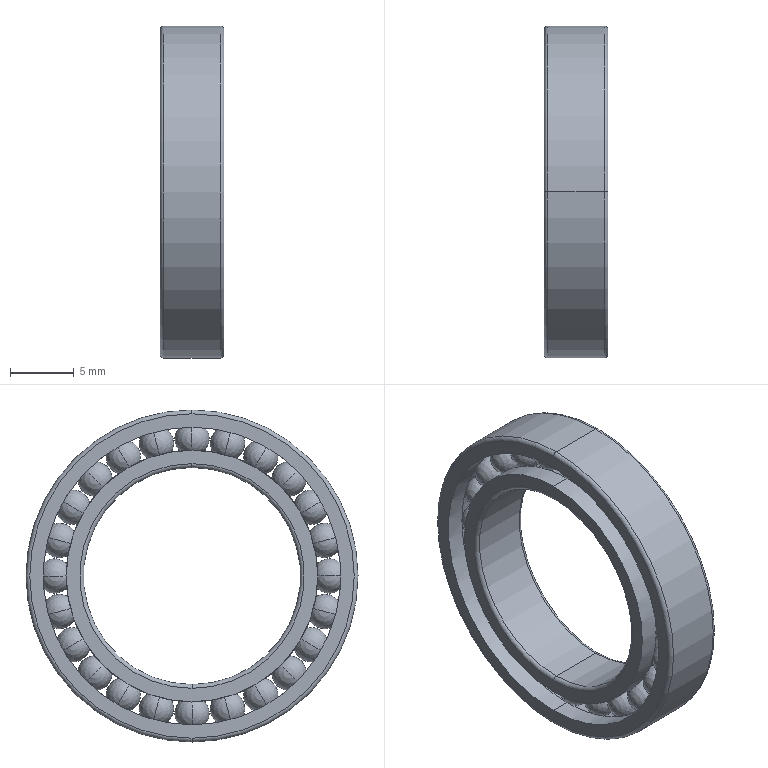Part | NX | features BREP 1 | 1 solid | 192 faces | box 5 x 26 x 26 mm | volume 1074 mm3 | sphere 96 | torus 80 | cylinder 12 | plane 4 | commonest cylinder face diameters 19.7 x4 23.3 x4 17 x2 26 x2